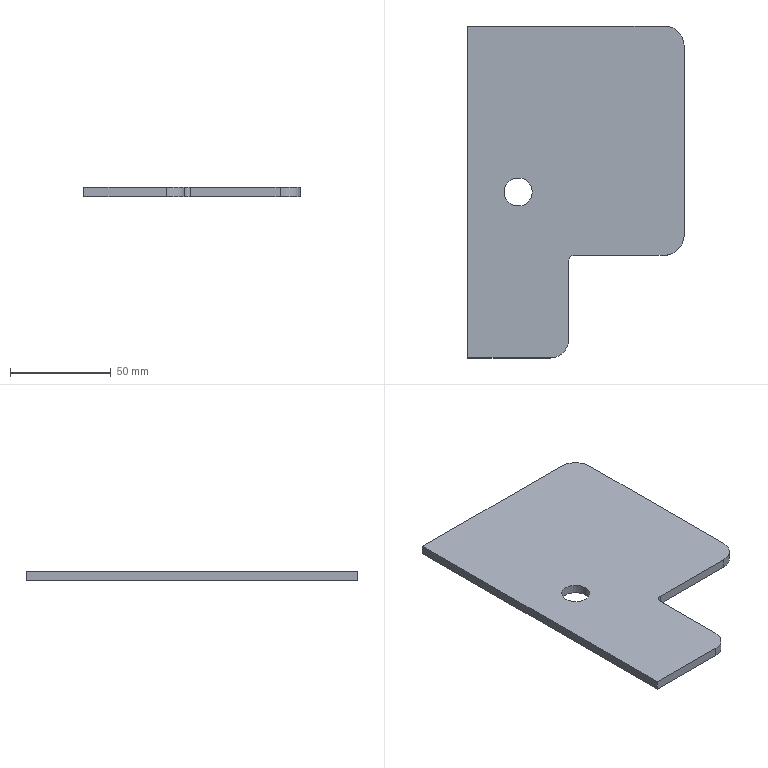Part | STEP file | DCV-000-013-B | 1 solid | 14 faces | box 107.5 x 165 x 4.5 mm | volume 65667 mm3 | plane 8 | cylinder 6 | commonest cylinder face diameters 14 x2 20 x2 6 x1 18 x1
STEP:
#1=CARTESIAN_POINT('',(0.,0.,0.));
#2=DIRECTION('',(0.,0.,1.));
#3=DIRECTION('',(1.,0.,0.));
#4=AXIS2_PLACEMENT_3D('',#1,#2,#3);
#5=CARTESIAN_POINT('',(32.,82.5,0.));
#6=VERTEX_POINT('',#5);
#7=CARTESIAN_POINT('',(32.,82.5,4.5));
#8=VERTEX_POINT('',#7);
#9=CARTESIAN_POINT('',(32.,82.5,-192.481));
#10=DIRECTION('',(0.,0.,1.));
#11=VECTOR('',#10,1.);
#12=LINE('',#9,#11);
#13=CARTESIAN_POINT('',(25.,82.5,-192.481));
#14=DIRECTION('',(0.,0.,1.));
#15=DIRECTION('',(1.,0.,0.));
#16=AXIS2_PLACEMENT_3D('',#13,#14,#15);
#17=CYLINDRICAL_SURFACE('',#16,7.);
#18=CARTESIAN_POINT('',(6.283,0.));
#19=DIRECTION('',(0.,1.));
#20=VECTOR('',#19,1.);
#21=LINE('',#18,#20);
#22=(GEOMETRIC_REPRESENTATION_CONTEXT(2)PARAMETRIC_REPRESENTATION_CONTEXT()REPRESENTATION_CONTEXT('',''));
#23=DEFINITIONAL_REPRESENTATION('',(#21),#22);
#24=PCURVE('',#17,#23);
#25=CARTESIAN_POINT('',(25.,82.5,-192.481));
#26=DIRECTION('',(0.,0.,1.));
#27=DIRECTION('',(1.,0.,0.));
#28=AXIS2_PLACEMENT_3D('',#25,#26,#27);
#29=CYLINDRICAL_SURFACE('',#28,7.);
#30=CARTESIAN_POINT('',(0.,0.));
#31=DIRECTION('',(0.,1.));
#32=VECTOR('',#31,1.);
#33=LINE('',#30,#32);
#34=(GEOMETRIC_REPRESENTATION_CONTEXT(2)PARAMETRIC_REPRESENTATION_CONTEXT()REPRESENTATION_CONTEXT('',''));
#35=DEFINITIONAL_REPRESENTATION('',(#33),#34);
#36=PCURVE('',#29,#35);
#37=SURFACE_CURVE('',#12,(#24,#36),.PCURVE_S1.);
#38=EDGE_CURVE('',#6,#8,#37,.T.);
#39=ORIENTED_EDGE('',*,*,#38,.T.);
#40=CARTESIAN_POINT('',(18.,82.5,4.5));
#41=VERTEX_POINT('',#40);
#42=CARTESIAN_POINT('',(25.,82.5,4.5));
#43=DIRECTION('',(0.,0.,-1.));
#44=DIRECTION('',(1.,0.,0.));
#45=AXIS2_PLACEMENT_3D('',#42,#43,#44);
#46=CIRCLE('',#45,7.);
#47=CARTESIAN_POINT('',(6.283,196.981));
#48=DIRECTION('',(-1.,0.));
#49=VECTOR('',#48,1.);
#50=LINE('',#47,#49);
#51=(GEOMETRIC_REPRESENTATION_CONTEXT(2)PARAMETRIC_REPRESENTATION_CONTEXT()REPRESENTATION_CONTEXT('',''));
#52=DEFINITIONAL_REPRESENTATION('',(#50),#51);
#53=PCURVE('',#17,#52);
#54=CARTESIAN_POINT('',(53.75,82.5,4.5));
#55=DIRECTION('',(0.,0.,1.));
#56=DIRECTION('',(1.,0.,0.));
#57=AXIS2_PLACEMENT_3D('',#54,#55,#56);
#58=PLANE('',#57);
#59=CARTESIAN_POINT('',(-21.75,0.));
#60=CARTESIAN_POINT('',(-21.75,-12.124));
#61=CARTESIAN_POINT('',(-32.25,-6.062));
#62=CARTESIAN_POINT('',(-42.75,0.));
#63=CARTESIAN_POINT('',(-32.25,6.062));
#64=CARTESIAN_POINT('',(-21.75,12.124));
#65=CARTESIAN_POINT('',(-21.75,0.));
#66=(BOUNDED_CURVE()B_SPLINE_CURVE(2,(#59,#60,#61,#62,#63,#64,#65),.UNSPECIFIED.,.T.,.F.)B_SPLINE_CURVE_WITH_KNOTS((1,2,2,2,2,1),(-2.094,0.,2.094,4.189,6.283,8.378),.UNSPECIFIED.)CURVE()GEOMETRIC_REPRESENTATION_ITEM()RATIONAL_B_SPLINE_CURVE((1.,0.5,1.,0.5,1.,0.5,1.))REPRESENTATION_ITEM(''));
#67=(GEOMETRIC_REPRESENTATION_CONTEXT(2)PARAMETRIC_REPRESENTATION_CONTEXT()REPRESENTATION_CONTEXT('',''));
#68=DEFINITIONAL_REPRESENTATION('',(#66),#67);
#69=PCURVE('',#58,#68);
#70=SURFACE_CURVE('',#46,(#53,#69),.PCURVE_S1.);
#71=EDGE_CURVE('',#8,#41,#70,.T.);
#72=ORIENTED_EDGE('',*,*,#71,.T.);
#73=CARTESIAN_POINT('',(18.,82.5,0.));
#74=VERTEX_POINT('',#73);
#75=CARTESIAN_POINT('',(18.,82.5,-192.481));
#76=DIRECTION('',(0.,0.,1.));
#77=VECTOR('',#76,1.);
#78=LINE('',#75,#77);
#79=CARTESIAN_POINT('',(3.142,0.));
#80=DIRECTION('',(0.,1.));
#81=VECTOR('',#80,1.);
#82=LINE('',#79,#81);
#83=(GEOMETRIC_REPRESENTATION_CONTEXT(2)PARAMETRIC_REPRESENTATION_CONTEXT()REPRESENTATION_CONTEXT('',''));
#84=DEFINITIONAL_REPRESENTATION('',(#82),#83);
#85=PCURVE('',#17,#84);
#86=CARTESIAN_POINT('',(3.142,0.));
#87=DIRECTION('',(0.,1.));
#88=VECTOR('',#87,1.);
#89=LINE('',#86,#88);
#90=(GEOMETRIC_REPRESENTATION_CONTEXT(2)PARAMETRIC_REPRESENTATION_CONTEXT()REPRESENTATION_CONTEXT('',''));
#91=DEFINITIONAL_REPRESENTATION('',(#89),#90);
#92=PCURVE('',#29,#91);
#93=SURFACE_CURVE('',#78,(#85,#92),.PCURVE_S1.);
#94=EDGE_CURVE('',#74,#41,#93,.T.);
#95=ORIENTED_EDGE('',*,*,#94,.F.);
#96=CARTESIAN_POINT('',(25.,82.5,0.));
#97=DIRECTION('',(0.,0.,1.));
#98=DIRECTION('',(1.,0.,0.));
#99=AXIS2_PLACEMENT_3D('',#96,#97,#98);
#100=CIRCLE('',#99,7.);
#101=CARTESIAN_POINT('',(0.,192.481));
#102=DIRECTION('',(1.,0.));
#103=VECTOR('',#102,1.);
#104=LINE('',#101,#103);
#105=(GEOMETRIC_REPRESENTATION_CONTEXT(2)PARAMETRIC_REPRESENTATION_CONTEXT()REPRESENTATION_CONTEXT('',''));
#106=DEFINITIONAL_REPRESENTATION('',(#104),#105);
#107=PCURVE('',#17,#106);
#108=CARTESIAN_POINT('',(53.75,82.5,0.));
#109=DIRECTION('',(0.,0.,1.));
#110=DIRECTION('',(1.,0.,0.));
#111=AXIS2_PLACEMENT_3D('',#108,#109,#110);
#112=PLANE('',#111);
#113=CARTESIAN_POINT('',(-28.75,0.));
#114=DIRECTION('',(1.,0.));
#115=AXIS2_PLACEMENT_2D('',#113,#114);
#116=CIRCLE('',#115,7.);
#117=(GEOMETRIC_REPRESENTATION_CONTEXT(2)PARAMETRIC_REPRESENTATION_CONTEXT()REPRESENTATION_CONTEXT('',''));
#118=DEFINITIONAL_REPRESENTATION('',(#116),#117);
#119=PCURVE('',#112,#118);
#120=SURFACE_CURVE('',#100,(#107,#119),.PCURVE_S1.);
#121=EDGE_CURVE('',#74,#6,#120,.T.);
#122=ORIENTED_EDGE('',*,*,#121,.T.);
#123=EDGE_LOOP('',(#39,#72,#95,#122));
#124=FACE_BOUND('',#123,.F.);
#125=ADVANCED_FACE('',(#124),#17,.F.);
#126=CARTESIAN_POINT('',(25.,82.5,0.));
#127=DIRECTION('',(0.,0.,1.));
#128=DIRECTION('',(1.,0.,0.));
#129=AXIS2_PLACEMENT_3D('',#126,#127,#128);
#130=CIRCLE('',#129,7.);
#131=CARTESIAN_POINT('',(-28.75,0.));
#132=DIRECTION('',(1.,0.));
#133=AXIS2_PLACEMENT_2D('',#131,#132);
#134=CIRCLE('',#133,7.);
#135=(GEOMETRIC_REPRESENTATION_CONTEXT(2)PARAMETRIC_REPRESENTATION_CONTEXT()REPRESENTATION_CONTEXT('',''));
#136=DEFINITIONAL_REPRESENTATION('',(#134),#135);
#137=PCURVE('',#112,#136);
#138=CARTESIAN_POINT('',(0.,192.481));
#139=DIRECTION('',(1.,0.));
#140=VECTOR('',#139,1.);
#141=LINE('',#138,#140);
#142=(GEOMETRIC_REPRESENTATION_CONTEXT(2)PARAMETRIC_REPRESENTATION_CONTEXT()REPRESENTATION_CONTEXT('',''));
#143=DEFINITIONAL_REPRESENTATION('',(#141),#142);
#144=PCURVE('',#29,#143);
#145=SURFACE_CURVE('',#130,(#137,#144),.PCURVE_S1.);
#146=EDGE_CURVE('',#6,#74,#145,.T.);
#147=ORIENTED_EDGE('',*,*,#146,.T.);
#148=ORIENTED_EDGE('',*,*,#121,.T.);
#149=EDGE_LOOP('',(#147,#148));
#150=FACE_BOUND('',#149,.T.);
#151=CARTESIAN_POINT('',(0.,165.,0.));
#152=VERTEX_POINT('',#151);
#153=CARTESIAN_POINT('',(0.,0.,0.));
#154=VERTEX_POINT('',#153);
#155=CARTESIAN_POINT('',(0.,165.,0.));
#156=DIRECTION('',(0.,-1.,0.));
#157=VECTOR('',#156,1.);
#158=LINE('',#155,#157);
#159=CARTESIAN_POINT('',(-53.75,82.5));
#160=DIRECTION('',(0.,-1.));
#161=VECTOR('',#160,1.);
#162=LINE('',#159,#161);
#163=(GEOMETRIC_REPRESENTATION_CONTEXT(2)PARAMETRIC_REPRESENTATION_CONTEXT()REPRESENTATION_CONTEXT('',''));
#164=DEFINITIONAL_REPRESENTATION('',(#162),#163);
#165=PCURVE('',#112,#164);
#166=CARTESIAN_POINT('',(0.,165.,0.));
#167=DIRECTION('',(-1.,0.,0.));
#168=DIRECTION('',(0.,0.,1.));
#169=AXIS2_PLACEMENT_3D('',#166,#167,#168);
#170=PLANE('',#169);
#171=CARTESIAN_POINT('',(0.,0.));
#172=DIRECTION('',(0.,-1.));
#173=VECTOR('',#172,1.);
#174=LINE('',#171,#173);
#175=(GEOMETRIC_REPRESENTATION_CONTEXT(2)PARAMETRIC_REPRESENTATION_CONTEXT()REPRESENTATION_CONTEXT('',''));
#176=DEFINITIONAL_REPRESENTATION('',(#174),#175);
#177=PCURVE('',#170,#176);
#178=SURFACE_CURVE('',#158,(#165,#177),.PCURVE_S1.);
#179=EDGE_CURVE('',#152,#154,#178,.T.);
#180=ORIENTED_EDGE('',*,*,#179,.F.);
#181=CARTESIAN_POINT('',(97.5,165.,0.));
#182=VERTEX_POINT('',#181);
#183=CARTESIAN_POINT('',(97.5,165.,0.));
#184=DIRECTION('',(-1.,0.,0.));
#185=VECTOR('',#184,1.);
#186=LINE('',#183,#185);
#187=CARTESIAN_POINT('',(43.75,82.5));
#188=DIRECTION('',(-1.,0.));
#189=VECTOR('',#188,1.);
#190=LINE('',#187,#189);
#191=(GEOMETRIC_REPRESENTATION_CONTEXT(2)PARAMETRIC_REPRESENTATION_CONTEXT()REPRESENTATION_CONTEXT('',''));
#192=DEFINITIONAL_REPRESENTATION('',(#190),#191);
#193=PCURVE('',#112,#192);
#194=CARTESIAN_POINT('',(97.5,165.,0.));
#195=DIRECTION('',(0.,1.,0.));
#196=DIRECTION('',(1.,0.,0.));
#197=AXIS2_PLACEMENT_3D('',#194,#195,#196);
#198=PLANE('',#197);
#199=CARTESIAN_POINT('',(0.,0.));
#200=DIRECTION('',(-1.,0.));
#201=VECTOR('',#200,1.);
#202=LINE('',#199,#201);
#203=(GEOMETRIC_REPRESENTATION_CONTEXT(2)PARAMETRIC_REPRESENTATION_CONTEXT()REPRESENTATION_CONTEXT('',''));
#204=DEFINITIONAL_REPRESENTATION('',(#202),#203);
#205=PCURVE('',#198,#204);
#206=SURFACE_CURVE('',#186,(#193,#205),.PCURVE_S1.);
#207=EDGE_CURVE('',#182,#152,#206,.T.);
#208=ORIENTED_EDGE('',*,*,#207,.F.);
#209=CARTESIAN_POINT('',(107.5,155.,0.));
#210=VERTEX_POINT('',#209);
#211=CARTESIAN_POINT('',(97.5,155.,0.));
#212=DIRECTION('',(0.,0.,1.));
#213=DIRECTION('',(1.,0.,0.));
#214=AXIS2_PLACEMENT_3D('',#211,#212,#213);
#215=CIRCLE('',#214,10.);
#216=CARTESIAN_POINT('',(43.75,72.5));
#217=DIRECTION('',(1.,0.));
#218=AXIS2_PLACEMENT_2D('',#216,#217);
#219=CIRCLE('',#218,10.);
#220=(GEOMETRIC_REPRESENTATION_CONTEXT(2)PARAMETRIC_REPRESENTATION_CONTEXT()REPRESENTATION_CONTEXT('',''));
#221=DEFINITIONAL_REPRESENTATION('',(#219),#220);
#222=PCURVE('',#112,#221);
#223=CARTESIAN_POINT('',(97.5,155.,0.));
#224=DIRECTION('',(0.,0.,1.));
#225=DIRECTION('',(1.,0.,0.));
#226=AXIS2_PLACEMENT_3D('',#223,#224,#225);
#227=CYLINDRICAL_SURFACE('',#226,10.);
#228=CARTESIAN_POINT('',(0.,0.));
#229=DIRECTION('',(1.,0.));
#230=VECTOR('',#229,1.);
#231=LINE('',#228,#230);
#232=(GEOMETRIC_REPRESENTATION_CONTEXT(2)PARAMETRIC_REPRESENTATION_CONTEXT()REPRESENTATION_CONTEXT('',''));
#233=DEFINITIONAL_REPRESENTATION('',(#231),#232);
#234=PCURVE('',#227,#233);
#235=SURFACE_CURVE('',#215,(#222,#234),.PCURVE_S1.);
#236=EDGE_CURVE('',#210,#182,#235,.T.);
#237=ORIENTED_EDGE('',*,*,#236,.F.);
#238=CARTESIAN_POINT('',(107.5,61.,0.));
#239=VERTEX_POINT('',#238);
#240=CARTESIAN_POINT('',(107.5,61.,0.));
#241=DIRECTION('',(0.,1.,0.));
#242=VECTOR('',#241,1.);
#243=LINE('',#240,#242);
#244=CARTESIAN_POINT('',(53.75,-21.5));
#245=DIRECTION('',(0.,1.));
#246=VECTOR('',#245,1.);
#247=LINE('',#244,#246);
#248=(GEOMETRIC_REPRESENTATION_CONTEXT(2)PARAMETRIC_REPRESENTATION_CONTEXT()REPRESENTATION_CONTEXT('',''));
#249=DEFINITIONAL_REPRESENTATION('',(#247),#248);
#250=PCURVE('',#112,#249);
#251=CARTESIAN_POINT('',(107.5,61.,0.));
#252=DIRECTION('',(1.,0.,0.));
#253=DIRECTION('',(0.,1.,0.));
#254=AXIS2_PLACEMENT_3D('',#251,#252,#253);
#255=PLANE('',#254);
#256=CARTESIAN_POINT('',(0.,0.));
#257=DIRECTION('',(1.,0.));
#258=VECTOR('',#257,1.);
#259=LINE('',#256,#258);
#260=(GEOMETRIC_REPRESENTATION_CONTEXT(2)PARAMETRIC_REPRESENTATION_CONTEXT()REPRESENTATION_CONTEXT('',''));
#261=DEFINITIONAL_REPRESENTATION('',(#259),#260);
#262=PCURVE('',#255,#261);
#263=SURFACE_CURVE('',#243,(#250,#262),.PCURVE_S1.);
#264=EDGE_CURVE('',#239,#210,#263,.T.);
#265=ORIENTED_EDGE('',*,*,#264,.F.);
#266=CARTESIAN_POINT('',(97.5,51.,0.));
#267=VERTEX_POINT('',#266);
#268=CARTESIAN_POINT('',(97.5,61.,0.));
#269=DIRECTION('',(0.,0.,1.));
#270=DIRECTION('',(0.,-1.,0.));
#271=AXIS2_PLACEMENT_3D('',#268,#269,#270);
#272=CIRCLE('',#271,10.);
#273=CARTESIAN_POINT('',(43.75,-21.5));
#274=DIRECTION('',(0.,-1.));
#275=AXIS2_PLACEMENT_2D('',#273,#274);
#276=CIRCLE('',#275,10.);
#277=(GEOMETRIC_REPRESENTATION_CONTEXT(2)PARAMETRIC_REPRESENTATION_CONTEXT()REPRESENTATION_CONTEXT('',''));
#278=DEFINITIONAL_REPRESENTATION('',(#276),#277);
#279=PCURVE('',#112,#278);
#280=CARTESIAN_POINT('',(97.5,61.,0.));
#281=DIRECTION('',(0.,0.,1.));
#282=DIRECTION('',(0.,-1.,0.));
#283=AXIS2_PLACEMENT_3D('',#280,#281,#282);
#284=CYLINDRICAL_SURFACE('',#283,10.);
#285=CARTESIAN_POINT('',(0.,0.));
#286=DIRECTION('',(1.,0.));
#287=VECTOR('',#286,1.);
#288=LINE('',#285,#287);
#289=(GEOMETRIC_REPRESENTATION_CONTEXT(2)PARAMETRIC_REPRESENTATION_CONTEXT()REPRESENTATION_CONTEXT('',''));
#290=DEFINITIONAL_REPRESENTATION('',(#288),#289);
#291=PCURVE('',#284,#290);
#292=SURFACE_CURVE('',#272,(#279,#291),.PCURVE_S1.);
#293=EDGE_CURVE('',#267,#239,#292,.T.);
#294=ORIENTED_EDGE('',*,*,#293,.F.);
#295=CARTESIAN_POINT('',(53.,51.,0.));
#296=VERTEX_POINT('',#295);
#297=CARTESIAN_POINT('',(53.,51.,0.));
#298=DIRECTION('',(1.,0.,0.));
#299=VECTOR('',#298,1.);
#300=LINE('',#297,#299);
#301=CARTESIAN_POINT('',(-0.75,-31.5));
#302=DIRECTION('',(1.,0.));
#303=VECTOR('',#302,1.);
#304=LINE('',#301,#303);
#305=(GEOMETRIC_REPRESENTATION_CONTEXT(2)PARAMETRIC_REPRESENTATION_CONTEXT()REPRESENTATION_CONTEXT('',''));
#306=DEFINITIONAL_REPRESENTATION('',(#304),#305);
#307=PCURVE('',#112,#306);
#308=CARTESIAN_POINT('',(53.,51.,0.));
#309=DIRECTION('',(0.,-1.,0.));
#310=DIRECTION('',(0.,0.,-1.));
#311=AXIS2_PLACEMENT_3D('',#308,#309,#310);
#312=PLANE('',#311);
#313=CARTESIAN_POINT('',(0.,0.));
#314=DIRECTION('',(0.,1.));
#315=VECTOR('',#314,1.);
#316=LINE('',#313,#315);
#317=(GEOMETRIC_REPRESENTATION_CONTEXT(2)PARAMETRIC_REPRESENTATION_CONTEXT()REPRESENTATION_CONTEXT('',''));
#318=DEFINITIONAL_REPRESENTATION('',(#316),#317);
#319=PCURVE('',#312,#318);
#320=SURFACE_CURVE('',#300,(#307,#319),.PCURVE_S1.);
#321=EDGE_CURVE('',#296,#267,#320,.T.);
#322=ORIENTED_EDGE('',*,*,#321,.F.);
#323=CARTESIAN_POINT('',(50.,48.,0.));
#324=VERTEX_POINT('',#323);
#325=CARTESIAN_POINT('',(53.,48.,0.));
#326=DIRECTION('',(0.,0.,-1.));
#327=DIRECTION('',(0.,-1.,0.));
#328=AXIS2_PLACEMENT_3D('',#325,#326,#327);
#329=CIRCLE('',#328,3.);
#330=CARTESIAN_POINT('',(-0.75,-37.5));
#331=CARTESIAN_POINT('',(-5.946,-37.5));
#332=CARTESIAN_POINT('',(-3.348,-33.));
#333=CARTESIAN_POINT('',(-0.75,-28.5));
#334=CARTESIAN_POINT('',(1.848,-33.));
#335=CARTESIAN_POINT('',(4.446,-37.5));
#336=CARTESIAN_POINT('',(-0.75,-37.5));
#337=(BOUNDED_CURVE()B_SPLINE_CURVE(2,(#330,#331,#332,#333,#334,#335,#336),.UNSPECIFIED.,.T.,.F.)B_SPLINE_CURVE_WITH_KNOTS((1,2,2,2,2,1),(-2.094,0.,2.094,4.189,6.283,8.378),.UNSPECIFIED.)CURVE()GEOMETRIC_REPRESENTATION_ITEM()RATIONAL_B_SPLINE_CURVE((1.,0.5,1.,0.5,1.,0.5,1.))REPRESENTATION_ITEM(''));
#338=(GEOMETRIC_REPRESENTATION_CONTEXT(2)PARAMETRIC_REPRESENTATION_CONTEXT()REPRESENTATION_CONTEXT('',''));
#339=DEFINITIONAL_REPRESENTATION('',(#337),#338);
#340=PCURVE('',#112,#339);
#341=CARTESIAN_POINT('',(53.,48.,0.));
#342=DIRECTION('',(0.,0.,1.));
#343=DIRECTION('',(0.,-1.,0.));
#344=AXIS2_PLACEMENT_3D('',#341,#342,#343);
#345=CYLINDRICAL_SURFACE('',#344,3.);
#346=CARTESIAN_POINT('',(6.283,0.));
#347=DIRECTION('',(-1.,0.));
#348=VECTOR('',#347,1.);
#349=LINE('',#346,#348);
#350=(GEOMETRIC_REPRESENTATION_CONTEXT(2)PARAMETRIC_REPRESENTATION_CONTEXT()REPRESENTATION_CONTEXT('',''));
#351=DEFINITIONAL_REPRESENTATION('',(#349),#350);
#352=PCURVE('',#345,#351);
#353=SURFACE_CURVE('',#329,(#340,#352),.PCURVE_S1.);
#354=EDGE_CURVE('',#324,#296,#353,.T.);
#355=ORIENTED_EDGE('',*,*,#354,.F.);
#356=CARTESIAN_POINT('',(50.,9.,0.));
#357=VERTEX_POINT('',#356);
#358=CARTESIAN_POINT('',(50.,9.,0.));
#359=DIRECTION('',(0.,1.,0.));
#360=VECTOR('',#359,1.);
#361=LINE('',#358,#360);
#362=CARTESIAN_POINT('',(-3.75,-73.5));
#363=DIRECTION('',(0.,1.));
#364=VECTOR('',#363,1.);
#365=LINE('',#362,#364);
#366=(GEOMETRIC_REPRESENTATION_CONTEXT(2)PARAMETRIC_REPRESENTATION_CONTEXT()REPRESENTATION_CONTEXT('',''));
#367=DEFINITIONAL_REPRESENTATION('',(#365),#366);
#368=PCURVE('',#112,#367);
#369=CARTESIAN_POINT('',(50.,9.,0.));
#370=DIRECTION('',(1.,0.,0.));
#371=DIRECTION('',(0.,1.,0.));
#372=AXIS2_PLACEMENT_3D('',#369,#370,#371);
#373=PLANE('',#372);
#374=CARTESIAN_POINT('',(0.,0.));
#375=DIRECTION('',(1.,0.));
#376=VECTOR('',#375,1.);
#377=LINE('',#374,#376);
#378=(GEOMETRIC_REPRESENTATION_CONTEXT(2)PARAMETRIC_REPRESENTATION_CONTEXT()REPRESENTATION_CONTEXT('',''));
#379=DEFINITIONAL_REPRESENTATION('',(#377),#378);
#380=PCURVE('',#373,#379);
#381=SURFACE_CURVE('',#361,(#368,#380),.PCURVE_S1.);
#382=EDGE_CURVE('',#357,#324,#381,.T.);
#383=ORIENTED_EDGE('',*,*,#382,.F.);
#384=CARTESIAN_POINT('',(41.,0.,0.));
#385=VERTEX_POINT('',#384);
#386=CARTESIAN_POINT('',(41.,9.,0.));
#387=DIRECTION('',(0.,0.,1.));
#388=DIRECTION('',(0.,-1.,0.));
#389=AXIS2_PLACEMENT_3D('',#386,#387,#388);
#390=CIRCLE('',#389,9.);
#391=CARTESIAN_POINT('',(-12.75,-73.5));
#392=DIRECTION('',(0.,-1.));
#393=AXIS2_PLACEMENT_2D('',#391,#392);
#394=CIRCLE('',#393,9.);
#395=(GEOMETRIC_REPRESENTATION_CONTEXT(2)PARAMETRIC_REPRESENTATION_CONTEXT()REPRESENTATION_CONTEXT('',''));
#396=DEFINITIONAL_REPRESENTATION('',(#394),#395);
#397=PCURVE('',#112,#396);
#398=CARTESIAN_POINT('',(41.,9.,0.));
#399=DIRECTION('',(0.,0.,1.));
#400=DIRECTION('',(0.,-1.,0.));
#401=AXIS2_PLACEMENT_3D('',#398,#399,#400);
#402=CYLINDRICAL_SURFACE('',#401,9.);
#403=CARTESIAN_POINT('',(0.,0.));
#404=DIRECTION('',(1.,0.));
#405=VECTOR('',#404,1.);
#406=LINE('',#403,#405);
#407=(GEOMETRIC_REPRESENTATION_CONTEXT(2)PARAMETRIC_REPRESENTATION_CONTEXT()REPRESENTATION_CONTEXT('',''));
#408=DEFINITIONAL_REPRESENTATION('',(#406),#407);
#409=PCURVE('',#402,#408);
#410=SURFACE_CURVE('',#390,(#397,#409),.PCURVE_S1.);
#411=EDGE_CURVE('',#385,#357,#410,.T.);
#412=ORIENTED_EDGE('',*,*,#411,.F.);
#413=CARTESIAN_POINT('',(0.,0.,0.));
#414=DIRECTION('',(1.,0.,0.));
#415=VECTOR('',#414,1.);
#416=LINE('',#413,#415);
#417=CARTESIAN_POINT('',(-53.75,-82.5));
#418=DIRECTION('',(1.,0.));
#419=VECTOR('',#418,1.);
#420=LINE('',#417,#419);
#421=(GEOMETRIC_REPRESENTATION_CONTEXT(2)PARAMETRIC_REPRESENTATION_CONTEXT()REPRESENTATION_CONTEXT('',''));
#422=DEFINITIONAL_REPRESENTATION('',(#420),#421);
#423=PCURVE('',#112,#422);
#424=CARTESIAN_POINT('',(0.,0.,0.));
#425=DIRECTION('',(0.,-1.,0.));
#426=DIRECTION('',(0.,0.,-1.));
#427=AXIS2_PLACEMENT_3D('',#424,#425,#426);
#428=PLANE('',#427);
#429=CARTESIAN_POINT('',(0.,0.));
#430=DIRECTION('',(0.,1.));
#431=VECTOR('',#430,1.);
#432=LINE('',#429,#431);
#433=(GEOMETRIC_REPRESENTATION_CONTEXT(2)PARAMETRIC_REPRESENTATION_CONTEXT()REPRESENTATION_CONTEXT('',''));
#434=DEFINITIONAL_REPRESENTATION('',(#432),#433);
#435=PCURVE('',#428,#434);
#436=SURFACE_CURVE('',#416,(#423,#435),.PCURVE_S1.);
#437=EDGE_CURVE('',#154,#385,#436,.T.);
#438=ORIENTED_EDGE('',*,*,#437,.F.);
#439=EDGE_LOOP('',(#180,#208,#237,#265,#294,#322,#355,#383,#412,#438));
#440=FACE_BOUND('',#439,.T.);
#441=ADVANCED_FACE('',(#150,#440),#112,.F.);
#442=ORIENTED_EDGE('',*,*,#71,.T.);
#443=CARTESIAN_POINT('',(25.,82.5,4.5));
#444=DIRECTION('',(0.,0.,-1.));
#445=DIRECTION('',(1.,0.,0.));
#446=AXIS2_PLACEMENT_3D('',#443,#444,#445);
#447=CIRCLE('',#446,7.);
#448=CARTESIAN_POINT('',(-21.75,0.));
#449=CARTESIAN_POINT('',(-21.75,-12.124));
#450=CARTESIAN_POINT('',(-32.25,-6.062));
#451=CARTESIAN_POINT('',(-42.75,0.));
#452=CARTESIAN_POINT('',(-32.25,6.062));
#453=CARTESIAN_POINT('',(-21.75,12.124));
#454=CARTESIAN_POINT('',(-21.75,0.));
#455=(BOUNDED_CURVE()B_SPLINE_CURVE(2,(#448,#449,#450,#451,#452,#453,#454),.UNSPECIFIED.,.T.,.F.)B_SPLINE_CURVE_WITH_KNOTS((1,2,2,2,2,1),(-2.094,0.,2.094,4.189,6.283,8.378),.UNSPECIFIED.)CURVE()GEOMETRIC_REPRESENTATION_ITEM()RATIONAL_B_SPLINE_CURVE((1.,0.5,1.,0.5,1.,0.5,1.))REPRESENTATION_ITEM(''));
#456=(GEOMETRIC_REPRESENTATION_CONTEXT(2)PARAMETRIC_REPRESENTATION_CONTEXT()REPRESENTATION_CONTEXT('',''));
#457=DEFINITIONAL_REPRESENTATION('',(#455),#456);
#458=PCURVE('',#58,#457);
#459=CARTESIAN_POINT('',(6.283,196.981));
#460=DIRECTION('',(-1.,0.));
#461=VECTOR('',#460,1.);
#462=LINE('',#459,#461);
#463=(GEOMETRIC_REPRESENTATION_CONTEXT(2)PARAMETRIC_REPRESENTATION_CONTEXT()REPRESENTATION_CONTEXT('',''));
#464=DEFINITIONAL_REPRESENTATION('',(#462),#463);
#465=PCURVE('',#29,#464);
#466=SURFACE_CURVE('',#447,(#458,#465),.PCURVE_S1.);
#467=EDGE_CURVE('',#41,#8,#466,.T.);
#468=ORIENTED_EDGE('',*,*,#467,.T.);
#469=EDGE_LOOP('',(#442,#468));
#470=FACE_BOUND('',#469,.T.);
#471=CARTESIAN_POINT('',(0.,165.,4.5));
#472=VERTEX_POINT('',#471);
#473=CARTESIAN_POINT('',(0.,0.,4.5));
#474=VERTEX_POINT('',#473);
#475=CARTESIAN_POINT('',(0.,165.,4.5));
#476=DIRECTION('',(0.,-1.,0.));
#477=VECTOR('',#476,1.);
#478=LINE('',#475,#477);
#479=CARTESIAN_POINT('',(-53.75,82.5));
#480=DIRECTION('',(0.,-1.));
#481=VECTOR('',#480,1.);
#482=LINE('',#479,#481);
#483=(GEOMETRIC_REPRESENTATION_CONTEXT(2)PARAMETRIC_REPRESENTATION_CONTEXT()REPRESENTATION_CONTEXT('',''));
#484=DEFINITIONAL_REPRESENTATION('',(#482),#483);
#485=PCURVE('',#58,#484);
#486=CARTESIAN_POINT('',(4.5,0.));
#487=DIRECTION('',(0.,-1.));
#488=VECTOR('',#487,1.);
#489=LINE('',#486,#488);
#490=(GEOMETRIC_REPRESENTATION_CONTEXT(2)PARAMETRIC_REPRESENTATION_CONTEXT()REPRESENTATION_CONTEXT('',''));
#491=DEFINITIONAL_REPRESENTATION('',(#489),#490);
#492=PCURVE('',#170,#491);
#493=SURFACE_CURVE('',#478,(#485,#492),.PCURVE_S1.);
#494=EDGE_CURVE('',#472,#474,#493,.T.);
#495=ORIENTED_EDGE('',*,*,#494,.T.);
#496=CARTESIAN_POINT('',(41.,0.,4.5));
#497=VERTEX_POINT('',#496);
#498=CARTESIAN_POINT('',(0.,0.,4.5));
#499=DIRECTION('',(1.,0.,0.));
#500=VECTOR('',#499,1.);
#501=LINE('',#498,#500);
#502=CARTESIAN_POINT('',(-53.75,-82.5));
#503=DIRECTION('',(1.,0.));
#504=VECTOR('',#503,1.);
#505=LINE('',#502,#504);
#506=(GEOMETRIC_REPRESENTATION_CONTEXT(2)PARAMETRIC_REPRESENTATION_CONTEXT()REPRESENTATION_CONTEXT('',''));
#507=DEFINITIONAL_REPRESENTATION('',(#505),#506);
#508=PCURVE('',#58,#507);
#509=CARTESIAN_POINT('',(-4.5,0.));
#510=DIRECTION('',(0.,1.));
#511=VECTOR('',#510,1.);
#512=LINE('',#509,#511);
#513=(GEOMETRIC_REPRESENTATION_CONTEXT(2)PARAMETRIC_REPRESENTATION_CONTEXT()REPRESENTATION_CONTEXT('',''));
#514=DEFINITIONAL_REPRESENTATION('',(#512),#513);
#515=PCURVE('',#428,#514);
#516=SURFACE_CURVE('',#501,(#508,#515),.PCURVE_S1.);
#517=EDGE_CURVE('',#474,#497,#516,.T.);
#518=ORIENTED_EDGE('',*,*,#517,.T.);
#519=CARTESIAN_POINT('',(50.,9.,4.5));
#520=VERTEX_POINT('',#519);
#521=CARTESIAN_POINT('',(41.,9.,4.5));
#522=DIRECTION('',(0.,0.,1.));
#523=DIRECTION('',(0.,-1.,0.));
#524=AXIS2_PLACEMENT_3D('',#521,#522,#523);
#525=CIRCLE('',#524,9.);
#526=CARTESIAN_POINT('',(-12.75,-73.5));
#527=DIRECTION('',(0.,-1.));
#528=AXIS2_PLACEMENT_2D('',#526,#527);
#529=CIRCLE('',#528,9.);
#530=(GEOMETRIC_REPRESENTATION_CONTEXT(2)PARAMETRIC_REPRESENTATION_CONTEXT()REPRESENTATION_CONTEXT('',''));
#531=DEFINITIONAL_REPRESENTATION('',(#529),#530);
#532=PCURVE('',#58,#531);
#533=CARTESIAN_POINT('',(0.,4.5));
#534=DIRECTION('',(1.,0.));
#535=VECTOR('',#534,1.);
#536=LINE('',#533,#535);
#537=(GEOMETRIC_REPRESENTATION_CONTEXT(2)PARAMETRIC_REPRESENTATION_CONTEXT()REPRESENTATION_CONTEXT('',''));
#538=DEFINITIONAL_REPRESENTATION('',(#536),#537);
#539=PCURVE('',#402,#538);
#540=SURFACE_CURVE('',#525,(#532,#539),.PCURVE_S1.);
#541=EDGE_CURVE('',#497,#520,#540,.T.);
#542=ORIENTED_EDGE('',*,*,#541,.T.);
#543=CARTESIAN_POINT('',(50.,48.,4.5));
#544=VERTEX_POINT('',#543);
#545=CARTESIAN_POINT('',(50.,9.,4.5));
#546=DIRECTION('',(0.,1.,0.));
#547=VECTOR('',#546,1.);
#548=LINE('',#545,#547);
#549=CARTESIAN_POINT('',(-3.75,-73.5));
#550=DIRECTION('',(0.,1.));
#551=VECTOR('',#550,1.);
#552=LINE('',#549,#551);
#553=(GEOMETRIC_REPRESENTATION_CONTEXT(2)PARAMETRIC_REPRESENTATION_CONTEXT()REPRESENTATION_CONTEXT('',''));
#554=DEFINITIONAL_REPRESENTATION('',(#552),#553);
#555=PCURVE('',#58,#554);
#556=CARTESIAN_POINT('',(0.,4.5));
#557=DIRECTION('',(1.,0.));
#558=VECTOR('',#557,1.);
#559=LINE('',#556,#558);
#560=(GEOMETRIC_REPRESENTATION_CONTEXT(2)PARAMETRIC_REPRESENTATION_CONTEXT()REPRESENTATION_CONTEXT('',''));
#561=DEFINITIONAL_REPRESENTATION('',(#559),#560);
#562=PCURVE('',#373,#561);
#563=SURFACE_CURVE('',#548,(#555,#562),.PCURVE_S1.);
#564=EDGE_CURVE('',#520,#544,#563,.T.);
#565=ORIENTED_EDGE('',*,*,#564,.T.);
#566=CARTESIAN_POINT('',(53.,51.,4.5));
#567=VERTEX_POINT('',#566);
#568=CARTESIAN_POINT('',(53.,48.,4.5));
#569=DIRECTION('',(0.,0.,-1.));
#570=DIRECTION('',(0.,-1.,0.));
#571=AXIS2_PLACEMENT_3D('',#568,#569,#570);
#572=CIRCLE('',#571,3.);
#573=CARTESIAN_POINT('',(-0.75,-37.5));
#574=CARTESIAN_POINT('',(-5.946,-37.5));
#575=CARTESIAN_POINT('',(-3.348,-33.));
#576=CARTESIAN_POINT('',(-0.75,-28.5));
#577=CARTESIAN_POINT('',(1.848,-33.));
#578=CARTESIAN_POINT('',(4.446,-37.5));
#579=CARTESIAN_POINT('',(-0.75,-37.5));
#580=(BOUNDED_CURVE()B_SPLINE_CURVE(2,(#573,#574,#575,#576,#577,#578,#579),.UNSPECIFIED.,.T.,.F.)B_SPLINE_CURVE_WITH_KNOTS((1,2,2,2,2,1),(-2.094,0.,2.094,4.189,6.283,8.378),.UNSPECIFIED.)CURVE()GEOMETRIC_REPRESENTATION_ITEM()RATIONAL_B_SPLINE_CURVE((1.,0.5,1.,0.5,1.,0.5,1.))REPRESENTATION_ITEM(''));
#581=(GEOMETRIC_REPRESENTATION_CONTEXT(2)PARAMETRIC_REPRESENTATION_CONTEXT()REPRESENTATION_CONTEXT('',''));
#582=DEFINITIONAL_REPRESENTATION('',(#580),#581);
#583=PCURVE('',#58,#582);
#584=CARTESIAN_POINT('',(6.283,4.5));
#585=DIRECTION('',(-1.,0.));
#586=VECTOR('',#585,1.);
#587=LINE('',#584,#586);
#588=(GEOMETRIC_REPRESENTATION_CONTEXT(2)PARAMETRIC_REPRESENTATION_CONTEXT()REPRESENTATION_CONTEXT('',''));
#589=DEFINITIONAL_REPRESENTATION('',(#587),#588);
#590=PCURVE('',#345,#589);
#591=SURFACE_CURVE('',#572,(#583,#590),.PCURVE_S1.);
#592=EDGE_CURVE('',#544,#567,#591,.T.);
#593=ORIENTED_EDGE('',*,*,#592,.T.);
#594=CARTESIAN_POINT('',(97.5,51.,4.5));
#595=VERTEX_POINT('',#594);
#596=CARTESIAN_POINT('',(53.,51.,4.5));
#597=DIRECTION('',(1.,0.,0.));
#598=VECTOR('',#597,1.);
#599=LINE('',#596,#598);
#600=CARTESIAN_POINT('',(-0.75,-31.5));
#601=DIRECTION('',(1.,0.));
#602=VECTOR('',#601,1.);
#603=LINE('',#600,#602);
#604=(GEOMETRIC_REPRESENTATION_CONTEXT(2)PARAMETRIC_REPRESENTATION_CONTEXT()REPRESENTATION_CONTEXT('',''));
#605=DEFINITIONAL_REPRESENTATION('',(#603),#604);
#606=PCURVE('',#58,#605);
#607=CARTESIAN_POINT('',(-4.5,0.));
#608=DIRECTION('',(0.,1.));
#609=VECTOR('',#608,1.);
#610=LINE('',#607,#609);
#611=(GEOMETRIC_REPRESENTATION_CONTEXT(2)PARAMETRIC_REPRESENTATION_CONTEXT()REPRESENTATION_CONTEXT('',''));
#612=DEFINITIONAL_REPRESENTATION('',(#610),#611);
#613=PCURVE('',#312,#612);
#614=SURFACE_CURVE('',#599,(#606,#613),.PCURVE_S1.);
#615=EDGE_CURVE('',#567,#595,#614,.T.);
#616=ORIENTED_EDGE('',*,*,#615,.T.);
#617=CARTESIAN_POINT('',(107.5,61.,4.5));
#618=VERTEX_POINT('',#617);
#619=CARTESIAN_POINT('',(97.5,61.,4.5));
#620=DIRECTION('',(0.,0.,1.));
#621=DIRECTION('',(0.,-1.,0.));
#622=AXIS2_PLACEMENT_3D('',#619,#620,#621);
#623=CIRCLE('',#622,10.);
#624=CARTESIAN_POINT('',(43.75,-21.5));
#625=DIRECTION('',(0.,-1.));
#626=AXIS2_PLACEMENT_2D('',#624,#625);
#627=CIRCLE('',#626,10.);
#628=(GEOMETRIC_REPRESENTATION_CONTEXT(2)PARAMETRIC_REPRESENTATION_CONTEXT()REPRESENTATION_CONTEXT('',''));
#629=DEFINITIONAL_REPRESENTATION('',(#627),#628);
#630=PCURVE('',#58,#629);
#631=CARTESIAN_POINT('',(0.,4.5));
#632=DIRECTION('',(1.,0.));
#633=VECTOR('',#632,1.);
#634=LINE('',#631,#633);
#635=(GEOMETRIC_REPRESENTATION_CONTEXT(2)PARAMETRIC_REPRESENTATION_CONTEXT()REPRESENTATION_CONTEXT('',''));
#636=DEFINITIONAL_REPRESENTATION('',(#634),#635);
#637=PCURVE('',#284,#636);
#638=SURFACE_CURVE('',#623,(#630,#637),.PCURVE_S1.);
#639=EDGE_CURVE('',#595,#618,#638,.T.);
#640=ORIENTED_EDGE('',*,*,#639,.T.);
#641=CARTESIAN_POINT('',(107.5,155.,4.5));
#642=VERTEX_POINT('',#641);
#643=CARTESIAN_POINT('',(107.5,61.,4.5));
#644=DIRECTION('',(0.,1.,0.));
#645=VECTOR('',#644,1.);
#646=LINE('',#643,#645);
#647=CARTESIAN_POINT('',(53.75,-21.5));
#648=DIRECTION('',(0.,1.));
#649=VECTOR('',#648,1.);
#650=LINE('',#647,#649);
#651=(GEOMETRIC_REPRESENTATION_CONTEXT(2)PARAMETRIC_REPRESENTATION_CONTEXT()REPRESENTATION_CONTEXT('',''));
#652=DEFINITIONAL_REPRESENTATION('',(#650),#651);
#653=PCURVE('',#58,#652);
#654=CARTESIAN_POINT('',(0.,4.5));
#655=DIRECTION('',(1.,0.));
#656=VECTOR('',#655,1.);
#657=LINE('',#654,#656);
#658=(GEOMETRIC_REPRESENTATION_CONTEXT(2)PARAMETRIC_REPRESENTATION_CONTEXT()REPRESENTATION_CONTEXT('',''));
#659=DEFINITIONAL_REPRESENTATION('',(#657),#658);
#660=PCURVE('',#255,#659);
#661=SURFACE_CURVE('',#646,(#653,#660),.PCURVE_S1.);
#662=EDGE_CURVE('',#618,#642,#661,.T.);
#663=ORIENTED_EDGE('',*,*,#662,.T.);
#664=CARTESIAN_POINT('',(97.5,165.,4.5));
#665=VERTEX_POINT('',#664);
#666=CARTESIAN_POINT('',(97.5,155.,4.5));
#667=DIRECTION('',(0.,0.,1.));
#668=DIRECTION('',(1.,0.,0.));
#669=AXIS2_PLACEMENT_3D('',#666,#667,#668);
#670=CIRCLE('',#669,10.);
#671=CARTESIAN_POINT('',(43.75,72.5));
#672=DIRECTION('',(1.,0.));
#673=AXIS2_PLACEMENT_2D('',#671,#672);
#674=CIRCLE('',#673,10.);
#675=(GEOMETRIC_REPRESENTATION_CONTEXT(2)PARAMETRIC_REPRESENTATION_CONTEXT()REPRESENTATION_CONTEXT('',''));
#676=DEFINITIONAL_REPRESENTATION('',(#674),#675);
#677=PCURVE('',#58,#676);
#678=CARTESIAN_POINT('',(0.,4.5));
#679=DIRECTION('',(1.,0.));
#680=VECTOR('',#679,1.);
#681=LINE('',#678,#680);
#682=(GEOMETRIC_REPRESENTATION_CONTEXT(2)PARAMETRIC_REPRESENTATION_CONTEXT()REPRESENTATION_CONTEXT('',''));
#683=DEFINITIONAL_REPRESENTATION('',(#681),#682);
#684=PCURVE('',#227,#683);
#685=SURFACE_CURVE('',#670,(#677,#684),.PCURVE_S1.);
#686=EDGE_CURVE('',#642,#665,#685,.T.);
#687=ORIENTED_EDGE('',*,*,#686,.T.);
#688=CARTESIAN_POINT('',(97.5,165.,4.5));
#689=DIRECTION('',(-1.,0.,0.));
#690=VECTOR('',#689,1.);
#691=LINE('',#688,#690);
#692=CARTESIAN_POINT('',(43.75,82.5));
#693=DIRECTION('',(-1.,0.));
#694=VECTOR('',#693,1.);
#695=LINE('',#692,#694);
#696=(GEOMETRIC_REPRESENTATION_CONTEXT(2)PARAMETRIC_REPRESENTATION_CONTEXT()REPRESENTATION_CONTEXT('',''));
#697=DEFINITIONAL_REPRESENTATION('',(#695),#696);
#698=PCURVE('',#58,#697);
#699=CARTESIAN_POINT('',(0.,-4.5));
#700=DIRECTION('',(-1.,0.));
#701=VECTOR('',#700,1.);
#702=LINE('',#699,#701);
#703=(GEOMETRIC_REPRESENTATION_CONTEXT(2)PARAMETRIC_REPRESENTATION_CONTEXT()REPRESENTATION_CONTEXT('',''));
#704=DEFINITIONAL_REPRESENTATION('',(#702),#703);
#705=PCURVE('',#198,#704);
#706=SURFACE_CURVE('',#691,(#698,#705),.PCURVE_S1.);
#707=EDGE_CURVE('',#665,#472,#706,.T.);
#708=ORIENTED_EDGE('',*,*,#707,.T.);
#709=EDGE_LOOP('',(#495,#518,#542,#565,#593,#616,#640,#663,#687,#708));
#710=FACE_BOUND('',#709,.T.);
#711=ADVANCED_FACE('',(#470,#710),#58,.T.);
#712=ORIENTED_EDGE('',*,*,#179,.T.);
#713=CARTESIAN_POINT('',(0.,0.,0.));
#714=DIRECTION('',(0.,0.,1.));
#715=VECTOR('',#714,1.);
#716=LINE('',#713,#715);
#717=CARTESIAN_POINT('',(0.,-165.));
#718=DIRECTION('',(1.,0.));
#719=VECTOR('',#718,1.);
#720=LINE('',#717,#719);
#721=(GEOMETRIC_REPRESENTATION_CONTEXT(2)PARAMETRIC_REPRESENTATION_CONTEXT()REPRESENTATION_CONTEXT('',''));
#722=DEFINITIONAL_REPRESENTATION('',(#720),#721);
#723=PCURVE('',#170,#722);
#724=CARTESIAN_POINT('',(0.,0.));
#725=DIRECTION('',(-1.,0.));
#726=VECTOR('',#725,1.);
#727=LINE('',#724,#726);
#728=(GEOMETRIC_REPRESENTATION_CONTEXT(2)PARAMETRIC_REPRESENTATION_CONTEXT()REPRESENTATION_CONTEXT('',''));
#729=DEFINITIONAL_REPRESENTATION('',(#727),#728);
#730=PCURVE('',#428,#729);
#731=SURFACE_CURVE('',#716,(#723,#730),.PCURVE_S1.);
#732=EDGE_CURVE('',#154,#474,#731,.T.);
#733=ORIENTED_EDGE('',*,*,#732,.T.);
#734=ORIENTED_EDGE('',*,*,#494,.F.);
#735=CARTESIAN_POINT('',(0.,165.,0.));
#736=DIRECTION('',(0.,0.,1.));
#737=VECTOR('',#736,1.);
#738=LINE('',#735,#737);
#739=CARTESIAN_POINT('',(0.,0.));
#740=DIRECTION('',(1.,0.));
#741=VECTOR('',#740,1.);
#742=LINE('',#739,#741);
#743=(GEOMETRIC_REPRESENTATION_CONTEXT(2)PARAMETRIC_REPRESENTATION_CONTEXT()REPRESENTATION_CONTEXT('',''));
#744=DEFINITIONAL_REPRESENTATION('',(#742),#743);
#745=PCURVE('',#170,#744);
#746=CARTESIAN_POINT('',(-97.5,0.));
#747=DIRECTION('',(0.,-1.));
#748=VECTOR('',#747,1.);
#749=LINE('',#746,#748);
#750=(GEOMETRIC_REPRESENTATION_CONTEXT(2)PARAMETRIC_REPRESENTATION_CONTEXT()REPRESENTATION_CONTEXT('',''));
#751=DEFINITIONAL_REPRESENTATION('',(#749),#750);
#752=PCURVE('',#198,#751);
#753=SURFACE_CURVE('',#738,(#745,#752),.PCURVE_S1.);
#754=EDGE_CURVE('',#152,#472,#753,.T.);
#755=ORIENTED_EDGE('',*,*,#754,.F.);
#756=EDGE_LOOP('',(#712,#733,#734,#755));
#757=FACE_BOUND('',#756,.T.);
#758=ADVANCED_FACE('',(#757),#170,.T.);
#759=ORIENTED_EDGE('',*,*,#437,.T.);
#760=CARTESIAN_POINT('',(41.,0.,0.));
#761=DIRECTION('',(0.,0.,1.));
#762=VECTOR('',#761,1.);
#763=LINE('',#760,#762);
#764=CARTESIAN_POINT('',(0.,41.));
#765=DIRECTION('',(-1.,0.));
#766=VECTOR('',#765,1.);
#767=LINE('',#764,#766);
#768=(GEOMETRIC_REPRESENTATION_CONTEXT(2)PARAMETRIC_REPRESENTATION_CONTEXT()REPRESENTATION_CONTEXT('',''));
#769=DEFINITIONAL_REPRESENTATION('',(#767),#768);
#770=PCURVE('',#428,#769);
#771=CARTESIAN_POINT('',(0.,0.));
#772=DIRECTION('',(0.,1.));
#773=VECTOR('',#772,1.);
#774=LINE('',#771,#773);
#775=(GEOMETRIC_REPRESENTATION_CONTEXT(2)PARAMETRIC_REPRESENTATION_CONTEXT()REPRESENTATION_CONTEXT('',''));
#776=DEFINITIONAL_REPRESENTATION('',(#774),#775);
#777=PCURVE('',#402,#776);
#778=SURFACE_CURVE('',#763,(#770,#777),.PCURVE_S1.);
#779=EDGE_CURVE('',#385,#497,#778,.T.);
#780=ORIENTED_EDGE('',*,*,#779,.T.);
#781=ORIENTED_EDGE('',*,*,#517,.F.);
#782=ORIENTED_EDGE('',*,*,#732,.F.);
#783=EDGE_LOOP('',(#759,#780,#781,#782));
#784=FACE_BOUND('',#783,.T.);
#785=ADVANCED_FACE('',(#784),#428,.T.);
#786=ORIENTED_EDGE('',*,*,#411,.T.);
#787=CARTESIAN_POINT('',(50.,9.,0.));
#788=DIRECTION('',(0.,0.,1.));
#789=VECTOR('',#788,1.);
#790=LINE('',#787,#789);
#791=CARTESIAN_POINT('',(1.571,0.));
#792=DIRECTION('',(0.,1.));
#793=VECTOR('',#792,1.);
#794=LINE('',#791,#793);
#795=(GEOMETRIC_REPRESENTATION_CONTEXT(2)PARAMETRIC_REPRESENTATION_CONTEXT()REPRESENTATION_CONTEXT('',''));
#796=DEFINITIONAL_REPRESENTATION('',(#794),#795);
#797=PCURVE('',#402,#796);
#798=CARTESIAN_POINT('',(0.,0.));
#799=DIRECTION('',(0.,1.));
#800=VECTOR('',#799,1.);
#801=LINE('',#798,#800);
#802=(GEOMETRIC_REPRESENTATION_CONTEXT(2)PARAMETRIC_REPRESENTATION_CONTEXT()REPRESENTATION_CONTEXT('',''));
#803=DEFINITIONAL_REPRESENTATION('',(#801),#802);
#804=PCURVE('',#373,#803);
#805=SURFACE_CURVE('',#790,(#797,#804),.PCURVE_S1.);
#806=EDGE_CURVE('',#357,#520,#805,.T.);
#807=ORIENTED_EDGE('',*,*,#806,.T.);
#808=ORIENTED_EDGE('',*,*,#541,.F.);
#809=ORIENTED_EDGE('',*,*,#779,.F.);
#810=EDGE_LOOP('',(#786,#807,#808,#809));
#811=FACE_BOUND('',#810,.T.);
#812=ADVANCED_FACE('',(#811),#402,.T.);
#813=ORIENTED_EDGE('',*,*,#382,.T.);
#814=CARTESIAN_POINT('',(50.,48.,0.));
#815=DIRECTION('',(0.,0.,1.));
#816=VECTOR('',#815,1.);
#817=LINE('',#814,#816);
#818=CARTESIAN_POINT('',(39.,0.));
#819=DIRECTION('',(0.,1.));
#820=VECTOR('',#819,1.);
#821=LINE('',#818,#820);
#822=(GEOMETRIC_REPRESENTATION_CONTEXT(2)PARAMETRIC_REPRESENTATION_CONTEXT()REPRESENTATION_CONTEXT('',''));
#823=DEFINITIONAL_REPRESENTATION('',(#821),#822);
#824=PCURVE('',#373,#823);
#825=CARTESIAN_POINT('',(4.712,0.));
#826=DIRECTION('',(0.,1.));
#827=VECTOR('',#826,1.);
#828=LINE('',#825,#827);
#829=(GEOMETRIC_REPRESENTATION_CONTEXT(2)PARAMETRIC_REPRESENTATION_CONTEXT()REPRESENTATION_CONTEXT('',''));
#830=DEFINITIONAL_REPRESENTATION('',(#828),#829);
#831=PCURVE('',#345,#830);
#832=SURFACE_CURVE('',#817,(#824,#831),.PCURVE_S1.);
#833=EDGE_CURVE('',#324,#544,#832,.T.);
#834=ORIENTED_EDGE('',*,*,#833,.T.);
#835=ORIENTED_EDGE('',*,*,#564,.F.);
#836=ORIENTED_EDGE('',*,*,#806,.F.);
#837=EDGE_LOOP('',(#813,#834,#835,#836));
#838=FACE_BOUND('',#837,.T.);
#839=ADVANCED_FACE('',(#838),#373,.T.);
#840=ORIENTED_EDGE('',*,*,#833,.T.);
#841=ORIENTED_EDGE('',*,*,#592,.T.);
#842=CARTESIAN_POINT('',(53.,51.,0.));
#843=DIRECTION('',(0.,0.,1.));
#844=VECTOR('',#843,1.);
#845=LINE('',#842,#844);
#846=CARTESIAN_POINT('',(3.142,0.));
#847=DIRECTION('',(0.,1.));
#848=VECTOR('',#847,1.);
#849=LINE('',#846,#848);
#850=(GEOMETRIC_REPRESENTATION_CONTEXT(2)PARAMETRIC_REPRESENTATION_CONTEXT()REPRESENTATION_CONTEXT('',''));
#851=DEFINITIONAL_REPRESENTATION('',(#849),#850);
#852=PCURVE('',#345,#851);
#853=CARTESIAN_POINT('',(0.,0.));
#854=DIRECTION('',(-1.,0.));
#855=VECTOR('',#854,1.);
#856=LINE('',#853,#855);
#857=(GEOMETRIC_REPRESENTATION_CONTEXT(2)PARAMETRIC_REPRESENTATION_CONTEXT()REPRESENTATION_CONTEXT('',''));
#858=DEFINITIONAL_REPRESENTATION('',(#856),#857);
#859=PCURVE('',#312,#858);
#860=SURFACE_CURVE('',#845,(#852,#859),.PCURVE_S1.);
#861=EDGE_CURVE('',#296,#567,#860,.T.);
#862=ORIENTED_EDGE('',*,*,#861,.F.);
#863=ORIENTED_EDGE('',*,*,#354,.F.);
#864=EDGE_LOOP('',(#840,#841,#862,#863));
#865=FACE_BOUND('',#864,.F.);
#866=ADVANCED_FACE('',(#865),#345,.F.);
#867=ORIENTED_EDGE('',*,*,#321,.T.);
#868=CARTESIAN_POINT('',(97.5,51.,0.));
#869=DIRECTION('',(0.,0.,1.));
#870=VECTOR('',#869,1.);
#871=LINE('',#868,#870);
#872=CARTESIAN_POINT('',(0.,44.5));
#873=DIRECTION('',(-1.,0.));
#874=VECTOR('',#873,1.);
#875=LINE('',#872,#874);
#876=(GEOMETRIC_REPRESENTATION_CONTEXT(2)PARAMETRIC_REPRESENTATION_CONTEXT()REPRESENTATION_CONTEXT('',''));
#877=DEFINITIONAL_REPRESENTATION('',(#875),#876);
#878=PCURVE('',#312,#877);
#879=CARTESIAN_POINT('',(0.,0.));
#880=DIRECTION('',(0.,1.));
#881=VECTOR('',#880,1.);
#882=LINE('',#879,#881);
#883=(GEOMETRIC_REPRESENTATION_CONTEXT(2)PARAMETRIC_REPRESENTATION_CONTEXT()REPRESENTATION_CONTEXT('',''));
#884=DEFINITIONAL_REPRESENTATION('',(#882),#883);
#885=PCURVE('',#284,#884);
#886=SURFACE_CURVE('',#871,(#878,#885),.PCURVE_S1.);
#887=EDGE_CURVE('',#267,#595,#886,.T.);
#888=ORIENTED_EDGE('',*,*,#887,.T.);
#889=ORIENTED_EDGE('',*,*,#615,.F.);
#890=ORIENTED_EDGE('',*,*,#861,.F.);
#891=EDGE_LOOP('',(#867,#888,#889,#890));
#892=FACE_BOUND('',#891,.T.);
#893=ADVANCED_FACE('',(#892),#312,.T.);
#894=ORIENTED_EDGE('',*,*,#293,.T.);
#895=CARTESIAN_POINT('',(107.5,61.,0.));
#896=DIRECTION('',(0.,0.,1.));
#897=VECTOR('',#896,1.);
#898=LINE('',#895,#897);
#899=CARTESIAN_POINT('',(1.571,0.));
#900=DIRECTION('',(0.,1.));
#901=VECTOR('',#900,1.);
#902=LINE('',#899,#901);
#903=(GEOMETRIC_REPRESENTATION_CONTEXT(2)PARAMETRIC_REPRESENTATION_CONTEXT()REPRESENTATION_CONTEXT('',''));
#904=DEFINITIONAL_REPRESENTATION('',(#902),#903);
#905=PCURVE('',#284,#904);
#906=CARTESIAN_POINT('',(0.,0.));
#907=DIRECTION('',(0.,1.));
#908=VECTOR('',#907,1.);
#909=LINE('',#906,#908);
#910=(GEOMETRIC_REPRESENTATION_CONTEXT(2)PARAMETRIC_REPRESENTATION_CONTEXT()REPRESENTATION_CONTEXT('',''));
#911=DEFINITIONAL_REPRESENTATION('',(#909),#910);
#912=PCURVE('',#255,#911);
#913=SURFACE_CURVE('',#898,(#905,#912),.PCURVE_S1.);
#914=EDGE_CURVE('',#239,#618,#913,.T.);
#915=ORIENTED_EDGE('',*,*,#914,.T.);
#916=ORIENTED_EDGE('',*,*,#639,.F.);
#917=ORIENTED_EDGE('',*,*,#887,.F.);
#918=EDGE_LOOP('',(#894,#915,#916,#917));
#919=FACE_BOUND('',#918,.T.);
#920=ADVANCED_FACE('',(#919),#284,.T.);
#921=ORIENTED_EDGE('',*,*,#264,.T.);
#922=CARTESIAN_POINT('',(107.5,155.,0.));
#923=DIRECTION('',(0.,0.,1.));
#924=VECTOR('',#923,1.);
#925=LINE('',#922,#924);
#926=CARTESIAN_POINT('',(94.,0.));
#927=DIRECTION('',(0.,1.));
#928=VECTOR('',#927,1.);
#929=LINE('',#926,#928);
#930=(GEOMETRIC_REPRESENTATION_CONTEXT(2)PARAMETRIC_REPRESENTATION_CONTEXT()REPRESENTATION_CONTEXT('',''));
#931=DEFINITIONAL_REPRESENTATION('',(#929),#930);
#932=PCURVE('',#255,#931);
#933=CARTESIAN_POINT('',(0.,0.));
#934=DIRECTION('',(0.,1.));
#935=VECTOR('',#934,1.);
#936=LINE('',#933,#935);
#937=(GEOMETRIC_REPRESENTATION_CONTEXT(2)PARAMETRIC_REPRESENTATION_CONTEXT()REPRESENTATION_CONTEXT('',''));
#938=DEFINITIONAL_REPRESENTATION('',(#936),#937);
#939=PCURVE('',#227,#938);
#940=SURFACE_CURVE('',#925,(#932,#939),.PCURVE_S1.);
#941=EDGE_CURVE('',#210,#642,#940,.T.);
#942=ORIENTED_EDGE('',*,*,#941,.T.);
#943=ORIENTED_EDGE('',*,*,#662,.F.);
#944=ORIENTED_EDGE('',*,*,#914,.F.);
#945=EDGE_LOOP('',(#921,#942,#943,#944));
#946=FACE_BOUND('',#945,.T.);
#947=ADVANCED_FACE('',(#946),#255,.T.);
#948=ORIENTED_EDGE('',*,*,#236,.T.);
#949=CARTESIAN_POINT('',(97.5,165.,0.));
#950=DIRECTION('',(0.,0.,1.));
#951=VECTOR('',#950,1.);
#952=LINE('',#949,#951);
#953=CARTESIAN_POINT('',(1.571,0.));
#954=DIRECTION('',(0.,1.));
#955=VECTOR('',#954,1.);
#956=LINE('',#953,#955);
#957=(GEOMETRIC_REPRESENTATION_CONTEXT(2)PARAMETRIC_REPRESENTATION_CONTEXT()REPRESENTATION_CONTEXT('',''));
#958=DEFINITIONAL_REPRESENTATION('',(#956),#957);
#959=PCURVE('',#227,#958);
#960=CARTESIAN_POINT('',(0.,0.));
#961=DIRECTION('',(0.,-1.));
#962=VECTOR('',#961,1.);
#963=LINE('',#960,#962);
#964=(GEOMETRIC_REPRESENTATION_CONTEXT(2)PARAMETRIC_REPRESENTATION_CONTEXT()REPRESENTATION_CONTEXT('',''));
#965=DEFINITIONAL_REPRESENTATION('',(#963),#964);
#966=PCURVE('',#198,#965);
#967=SURFACE_CURVE('',#952,(#959,#966),.PCURVE_S1.);
#968=EDGE_CURVE('',#182,#665,#967,.T.);
#969=ORIENTED_EDGE('',*,*,#968,.T.);
#970=ORIENTED_EDGE('',*,*,#686,.F.);
#971=ORIENTED_EDGE('',*,*,#941,.F.);
#972=EDGE_LOOP('',(#948,#969,#970,#971));
#973=FACE_BOUND('',#972,.T.);
#974=ADVANCED_FACE('',(#973),#227,.T.);
#975=ORIENTED_EDGE('',*,*,#207,.T.);
#976=ORIENTED_EDGE('',*,*,#754,.T.);
#977=ORIENTED_EDGE('',*,*,#707,.F.);
#978=ORIENTED_EDGE('',*,*,#968,.F.);
#979=EDGE_LOOP('',(#975,#976,#977,#978));
#980=FACE_BOUND('',#979,.T.);
#981=ADVANCED_FACE('',(#980),#198,.T.);
#982=ORIENTED_EDGE('',*,*,#467,.T.);
#983=ORIENTED_EDGE('',*,*,#38,.F.);
#984=ORIENTED_EDGE('',*,*,#146,.T.);
#985=ORIENTED_EDGE('',*,*,#94,.T.);
#986=EDGE_LOOP('',(#982,#983,#984,#985));
#987=FACE_BOUND('',#986,.F.);
#988=ADVANCED_FACE('',(#987),#29,.F.);
#989=CLOSED_SHELL('',(#125,#441,#711,#758,#785,#812,#839,#866,#893,#920,#947,#974,#981,#988));
#990=MANIFOLD_SOLID_BREP('',#989);
#991=(LENGTH_UNIT()NAMED_UNIT(*)SI_UNIT(.MILLI.,.METRE.));
#992=UNCERTAINTY_MEASURE_WITH_UNIT(LENGTH_MEASURE(0.0000001),#991,'','');
#993=(NAMED_UNIT(*)PLANE_ANGLE_UNIT()SI_UNIT($,.RADIAN.));
#994=(NAMED_UNIT(*)SI_UNIT($,.STERADIAN.)SOLID_ANGLE_UNIT());
#995=(GEOMETRIC_REPRESENTATION_CONTEXT(3)GLOBAL_UNCERTAINTY_ASSIGNED_CONTEXT((#992))GLOBAL_UNIT_ASSIGNED_CONTEXT((#991,#993,#994))REPRESENTATION_CONTEXT('',''));
#996=ADVANCED_BREP_SHAPE_REPRESENTATION('',(#4,#990),#995);